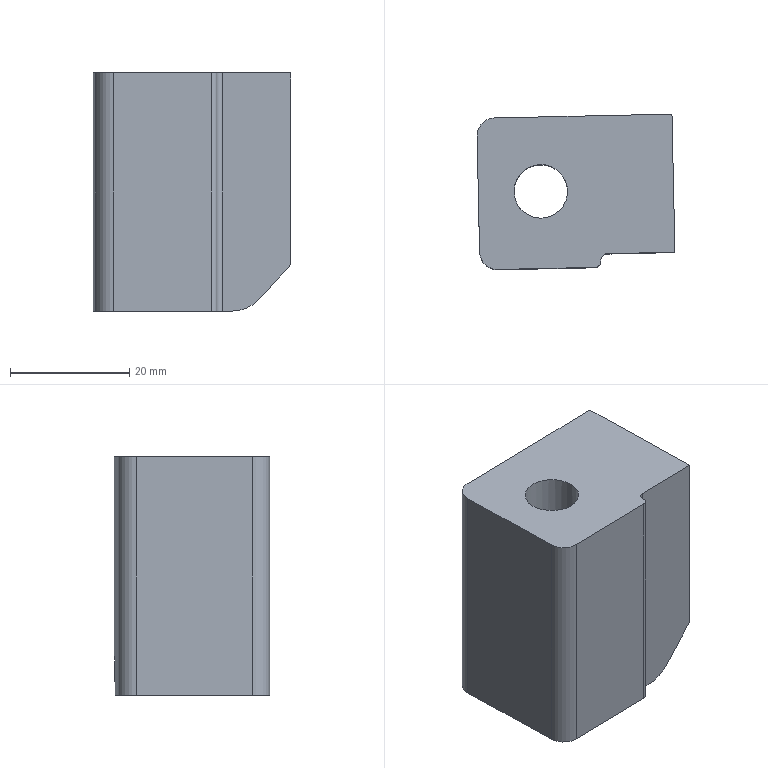Part | NX | features PS-18 2 | 1 solid | 17 faces | box 33.246 x 26.101 x 40 mm | volume 27415 mm3 | plane 10 | cylinder 7 | commonest cylinder face diameters 6.02 x2 1.98 x1 2.02 x1 9 x1 12 x1 14.5 x1
STEP:
#1=CARTESIAN_POINT('',(3013.955,-811.524,860.716));
#2=VERTEX_POINT('',#1);
#3=CARTESIAN_POINT('',(3006.705,-811.524,860.716));
#4=DIRECTION('',(0.,0.,1.));
#5=DIRECTION('',(1.,0.,0.));
#6=AXIS2_PLACEMENT_3D('',#3,#4,#5);
#7=CIRCLE('',#6,7.25);
#8=EDGE_CURVE('',#2,#2,#7,.T.);
#9=ORIENTED_EDGE('',*,*,#8,.T.);
#10=EDGE_LOOP('',(#9));
#11=FACE_BOUND('',#10,.T.);
#12=CARTESIAN_POINT('',(3016.814,-823.258,860.716));
#13=VERTEX_POINT('',#12);
#14=CARTESIAN_POINT('',(3016.809,-823.002,860.716));
#15=VERTEX_POINT('',#14);
#16=CARTESIAN_POINT('',(3016.836,-824.258,860.716));
#17=DIRECTION('',(0.0214,-0.9998,0.));
#18=VECTOR('',#17,1000.);
#19=LINE('',#16,#18);
#20=EDGE_CURVE('',#13,#15,#19,.F.);
#21=ORIENTED_EDGE('',*,*,#20,.F.);
#22=CARTESIAN_POINT('',(3015.826,-824.29,860.716));
#23=VERTEX_POINT('',#22);
#24=CARTESIAN_POINT('',(3015.804,-823.28,860.716));
#25=DIRECTION('',(0.,0.,1.));
#26=DIRECTION('',(1.,0.,0.));
#27=AXIS2_PLACEMENT_3D('',#24,#25,#26);
#28=CIRCLE('',#27,1.01);
#29=EDGE_CURVE('',#13,#23,#28,.F.);
#30=ORIENTED_EDGE('',*,*,#29,.T.);
#31=CARTESIAN_POINT('',(2999.484,-824.639,860.716));
#32=VERTEX_POINT('',#31);
#33=CARTESIAN_POINT('',(2866.42,-827.487,860.716));
#34=DIRECTION('',(0.9998,0.0214,0.));
#35=VECTOR('',#34,1000.);
#36=LINE('',#33,#35);
#37=EDGE_CURVE('',#23,#32,#36,.F.);
#38=ORIENTED_EDGE('',*,*,#37,.T.);
#39=CARTESIAN_POINT('',(2996.411,-821.694,860.716));
#40=VERTEX_POINT('',#39);
#41=CARTESIAN_POINT('',(2999.42,-821.63,860.716));
#42=DIRECTION('',(0.,0.,1.));
#43=DIRECTION('',(1.,0.,0.));
#44=AXIS2_PLACEMENT_3D('',#41,#42,#43);
#45=CIRCLE('',#44,3.01);
#46=EDGE_CURVE('',#32,#40,#45,.F.);
#47=ORIENTED_EDGE('',*,*,#46,.T.);
#48=CARTESIAN_POINT('',(2995.994,-802.251,860.716));
#49=VERTEX_POINT('',#48);
#50=CARTESIAN_POINT('',(2995.93,-799.251,860.716));
#51=DIRECTION('',(0.0214,-0.9998,0.));
#52=VECTOR('',#51,1000.);
#53=LINE('',#50,#52);
#54=EDGE_CURVE('',#49,#40,#53,.T.);
#55=ORIENTED_EDGE('',*,*,#54,.F.);
#56=CARTESIAN_POINT('',(2998.939,-799.177,860.716));
#57=VERTEX_POINT('',#56);
#58=CARTESIAN_POINT('',(2999.004,-802.186,860.716));
#59=DIRECTION('',(0.,0.,1.));
#60=DIRECTION('',(1.,0.,0.));
#61=AXIS2_PLACEMENT_3D('',#58,#59,#60);
#62=CIRCLE('',#61,3.01);
#63=EDGE_CURVE('',#49,#57,#62,.F.);
#64=ORIENTED_EDGE('',*,*,#63,.T.);
#65=CARTESIAN_POINT('',(3018.912,-798.75,860.716));
#66=VERTEX_POINT('',#65);
#67=CARTESIAN_POINT('',(3028.943,-798.535,860.716));
#68=DIRECTION('',(-0.9998,-0.0214,0.));
#69=VECTOR('',#68,1000.);
#70=LINE('',#67,#69);
#71=EDGE_CURVE('',#57,#66,#70,.F.);
#72=ORIENTED_EDGE('',*,*,#71,.T.);
#73=CARTESIAN_POINT('',(3019.409,-821.956,860.716));
#74=VERTEX_POINT('',#73);
#75=CARTESIAN_POINT('',(3023.131,-995.847,860.716));
#76=DIRECTION('',(0.0214,-0.9998,0.));
#77=VECTOR('',#76,1000.);
#78=LINE('',#75,#77);
#79=EDGE_CURVE('',#66,#74,#78,.T.);
#80=ORIENTED_EDGE('',*,*,#79,.T.);
#81=CARTESIAN_POINT('',(3017.777,-821.991,860.716));
#82=VERTEX_POINT('',#81);
#83=CARTESIAN_POINT('',(2866.372,-825.232,860.716));
#84=DIRECTION('',(0.9998,0.0214,0.));
#85=VECTOR('',#84,1000.);
#86=LINE('',#83,#85);
#87=EDGE_CURVE('',#74,#82,#86,.F.);
#88=ORIENTED_EDGE('',*,*,#87,.T.);
#89=CARTESIAN_POINT('',(3017.798,-822.981,860.716));
#90=DIRECTION('',(0.,0.,1.));
#91=DIRECTION('',(1.,0.,0.));
#92=AXIS2_PLACEMENT_3D('',#89,#90,#91);
#93=CIRCLE('',#92,0.99);
#94=EDGE_CURVE('',#82,#15,#93,.T.);
#95=ORIENTED_EDGE('',*,*,#94,.T.);
#96=EDGE_LOOP('',(#21,#30,#38,#47,#55,#64,#72,#80,#88,#95));
#97=FACE_BOUND('',#96,.T.);
#98=CARTESIAN_POINT('',(2870.094,-999.122,860.716));
#99=DIRECTION('',(0.,0.,1.));
#100=DIRECTION('',(0.,1.,0.));
#101=AXIS2_PLACEMENT_3D('',#98,#99,#100);
#102=PLANE('',#101);
#103=ADVANCED_FACE('',(#11,#97),#102,.F.);
#104=ORIENTED_EDGE('',*,*,#20,.T.);
#105=CARTESIAN_POINT('',(3016.809,-823.002,900.716));
#106=VERTEX_POINT('',#105);
#107=CARTESIAN_POINT('',(3016.809,-823.002,880.716));
#108=DIRECTION('',(0.,0.,1.));
#109=VECTOR('',#108,1000.);
#110=LINE('',#107,#109);
#111=EDGE_CURVE('',#15,#106,#110,.T.);
#112=ORIENTED_EDGE('',*,*,#111,.T.);
#113=CARTESIAN_POINT('',(3016.814,-823.258,900.716));
#114=VERTEX_POINT('',#113);
#115=CARTESIAN_POINT('',(3016.836,-824.258,900.716));
#116=DIRECTION('',(0.0214,-0.9998,0.));
#117=VECTOR('',#116,1000.);
#118=LINE('',#115,#117);
#119=EDGE_CURVE('',#106,#114,#118,.T.);
#120=ORIENTED_EDGE('',*,*,#119,.T.);
#121=CARTESIAN_POINT('',(3016.814,-823.258,880.716));
#122=DIRECTION('',(0.,0.,1.));
#123=VECTOR('',#122,1000.);
#124=LINE('',#121,#123);
#125=EDGE_CURVE('',#114,#13,#124,.F.);
#126=ORIENTED_EDGE('',*,*,#125,.T.);
#127=EDGE_LOOP('',(#104,#112,#120,#126));
#128=FACE_BOUND('',#127,.T.);
#129=CARTESIAN_POINT('',(3016.836,-824.258,880.716));
#130=DIRECTION('',(0.9998,0.0214,0.));
#131=DIRECTION('',(0.,0.,1.));
#132=AXIS2_PLACEMENT_3D('',#129,#130,#131);
#133=PLANE('',#132);
#134=ADVANCED_FACE('',(#128),#133,.T.);
#135=ORIENTED_EDGE('',*,*,#37,.F.);
#136=CARTESIAN_POINT('',(3015.826,-824.29,900.716));
#137=VERTEX_POINT('',#136);
#138=CARTESIAN_POINT('',(3015.826,-824.29,880.716));
#139=DIRECTION('',(0.,0.,-1.));
#140=VECTOR('',#139,1000.);
#141=LINE('',#138,#140);
#142=EDGE_CURVE('',#23,#137,#141,.F.);
#143=ORIENTED_EDGE('',*,*,#142,.T.);
#144=CARTESIAN_POINT('',(2999.484,-824.639,900.716));
#145=VERTEX_POINT('',#144);
#146=CARTESIAN_POINT('',(2881.104,-827.173,900.716));
#147=DIRECTION('',(0.9998,0.0214,0.));
#148=VECTOR('',#147,1000.);
#149=LINE('',#146,#148);
#150=EDGE_CURVE('',#145,#137,#149,.T.);
#151=ORIENTED_EDGE('',*,*,#150,.F.);
#152=CARTESIAN_POINT('',(2999.484,-824.639,880.716));
#153=DIRECTION('',(0.,0.,-1.));
#154=VECTOR('',#153,1000.);
#155=LINE('',#152,#154);
#156=EDGE_CURVE('',#145,#32,#155,.T.);
#157=ORIENTED_EDGE('',*,*,#156,.T.);
#158=EDGE_LOOP('',(#135,#143,#151,#157));
#159=FACE_BOUND('',#158,.T.);
#160=CARTESIAN_POINT('',(2996.485,-824.703,880.716));
#161=DIRECTION('',(0.0214,-0.9998,0.));
#162=DIRECTION('',(0.,0.,-1.));
#163=AXIS2_PLACEMENT_3D('',#160,#161,#162);
#164=PLANE('',#163);
#165=ADVANCED_FACE('',(#159),#164,.T.);
#166=CARTESIAN_POINT('',(2995.994,-802.251,900.716));
#167=VERTEX_POINT('',#166);
#168=CARTESIAN_POINT('',(2996.411,-821.694,900.716));
#169=VERTEX_POINT('',#168);
#170=CARTESIAN_POINT('',(2995.295,-769.576,900.716));
#171=DIRECTION('',(-0.0214,0.9998,0.));
#172=VECTOR('',#171,1000.);
#173=LINE('',#170,#172);
#174=EDGE_CURVE('',#167,#169,#173,.F.);
#175=ORIENTED_EDGE('',*,*,#174,.F.);
#176=CARTESIAN_POINT('',(2995.994,-802.251,888.716));
#177=DIRECTION('',(0.,0.,1.));
#178=VECTOR('',#177,1000.);
#179=LINE('',#176,#178);
#180=EDGE_CURVE('',#167,#49,#179,.F.);
#181=ORIENTED_EDGE('',*,*,#180,.T.);
#182=ORIENTED_EDGE('',*,*,#54,.T.);
#183=CARTESIAN_POINT('',(2996.411,-821.694,888.716));
#184=DIRECTION('',(0.,0.,1.));
#185=VECTOR('',#184,1000.);
#186=LINE('',#183,#185);
#187=EDGE_CURVE('',#40,#169,#186,.T.);
#188=ORIENTED_EDGE('',*,*,#187,.T.);
#189=EDGE_LOOP('',(#175,#181,#182,#188));
#190=FACE_BOUND('',#189,.T.);
#191=CARTESIAN_POINT('',(2995.93,-799.251,888.716));
#192=DIRECTION('',(0.9998,0.0214,0.));
#193=DIRECTION('',(0.,0.,1.));
#194=AXIS2_PLACEMENT_3D('',#191,#192,#193);
#195=PLANE('',#194);
#196=ADVANCED_FACE('',(#190),#195,.F.);
#197=ORIENTED_EDGE('',*,*,#71,.F.);
#198=CARTESIAN_POINT('',(2998.939,-799.177,900.716));
#199=VERTEX_POINT('',#198);
#200=CARTESIAN_POINT('',(2998.939,-799.177,888.716));
#201=DIRECTION('',(0.,0.,-1.));
#202=VECTOR('',#201,1000.);
#203=LINE('',#200,#202);
#204=EDGE_CURVE('',#57,#199,#203,.F.);
#205=ORIENTED_EDGE('',*,*,#204,.T.);
#206=CARTESIAN_POINT('',(3020.228,-798.721,900.716));
#207=VERTEX_POINT('',#206);
#208=CARTESIAN_POINT('',(2880.559,-801.711,900.716));
#209=DIRECTION('',(0.9998,0.0214,0.));
#210=VECTOR('',#209,1000.);
#211=LINE('',#208,#210);
#212=EDGE_CURVE('',#199,#207,#211,.T.);
#213=ORIENTED_EDGE('',*,*,#212,.T.);
#214=CARTESIAN_POINT('',(3026.717,-798.583,900.716));
#215=VERTEX_POINT('',#214);
#216=CARTESIAN_POINT('',(2880.559,-801.711,900.716));
#217=DIRECTION('',(0.9998,0.0214,0.));
#218=VECTOR('',#217,1000.);
#219=LINE('',#216,#218);
#220=EDGE_CURVE('',#207,#215,#219,.T.);
#221=ORIENTED_EDGE('',*,*,#220,.T.);
#222=CARTESIAN_POINT('',(3028.743,-798.539,900.716));
#223=VERTEX_POINT('',#222);
#224=CARTESIAN_POINT('',(2880.559,-801.711,900.716));
#225=DIRECTION('',(0.9998,0.0214,0.));
#226=VECTOR('',#225,1000.);
#227=LINE('',#224,#226);
#228=EDGE_CURVE('',#215,#223,#227,.T.);
#229=ORIENTED_EDGE('',*,*,#228,.T.);
#230=CARTESIAN_POINT('',(3028.743,-798.539,868.5));
#231=VERTEX_POINT('',#230);
#232=CARTESIAN_POINT('',(3028.743,-798.539,888.716));
#233=DIRECTION('',(0.,0.,1.));
#234=VECTOR('',#233,1000.);
#235=LINE('',#232,#234);
#236=EDGE_CURVE('',#223,#231,#235,.F.);
#237=ORIENTED_EDGE('',*,*,#236,.T.);
#238=CARTESIAN_POINT('',(3023.313,-798.655,862.638));
#239=VERTEX_POINT('',#238);
#240=CARTESIAN_POINT('',(3024.151,-798.637,863.544));
#241=DIRECTION('',(0.6795,0.01454,0.7335));
#242=VECTOR('',#241,1000.);
#243=LINE('',#240,#242);
#244=EDGE_CURVE('',#231,#239,#243,.F.);
#245=ORIENTED_EDGE('',*,*,#244,.T.);
#246=CARTESIAN_POINT('',(3018.912,-798.75,866.716));
#247=DIRECTION('',(0.0214,-0.9998,0.));
#248=DIRECTION('',(0.9998,0.0214,0.));
#249=AXIS2_PLACEMENT_3D('',#246,#247,#248);
#250=CIRCLE('',#249,6.);
#251=EDGE_CURVE('',#239,#66,#250,.F.);
#252=ORIENTED_EDGE('',*,*,#251,.T.);
#253=EDGE_LOOP('',(#197,#205,#213,#221,#229,#237,#245,#252));
#254=FACE_BOUND('',#253,.T.);
#255=CARTESIAN_POINT('',(3028.943,-798.535,888.716));
#256=DIRECTION('',(0.0214,-0.9998,0.));
#257=DIRECTION('',(0.,0.,1.));
#258=AXIS2_PLACEMENT_3D('',#255,#256,#257);
#259=PLANE('',#258);
#260=ADVANCED_FACE('',(#254),#259,.F.);
#261=ORIENTED_EDGE('',*,*,#251,.F.);
#262=CARTESIAN_POINT('',(3023.809,-821.862,862.638));
#263=VERTEX_POINT('',#262);
#264=CARTESIAN_POINT('',(3023.521,-808.389,862.638));
#265=DIRECTION('',(0.0214,-0.9998,0.));
#266=VECTOR('',#265,1000.);
#267=LINE('',#264,#266);
#268=EDGE_CURVE('',#263,#239,#267,.F.);
#269=ORIENTED_EDGE('',*,*,#268,.F.);
#270=CARTESIAN_POINT('',(3019.409,-821.956,866.716));
#271=DIRECTION('',(0.0214,-0.9998,0.));
#272=DIRECTION('',(0.9998,0.0214,0.));
#273=AXIS2_PLACEMENT_3D('',#270,#271,#272);
#274=CIRCLE('',#273,6.);
#275=EDGE_CURVE('',#74,#263,#274,.T.);
#276=ORIENTED_EDGE('',*,*,#275,.F.);
#277=ORIENTED_EDGE('',*,*,#79,.F.);
#278=EDGE_LOOP('',(#261,#269,#276,#277));
#279=FACE_BOUND('',#278,.T.);
#280=CARTESIAN_POINT('',(3023.131,-995.847,866.716));
#281=DIRECTION('',(0.0214,-0.9998,0.));
#282=DIRECTION('',(0.9998,0.0214,0.));
#283=AXIS2_PLACEMENT_3D('',#280,#281,#282);
#284=CYLINDRICAL_SURFACE('',#283,6.);
#285=ADVANCED_FACE('',(#279),#284,.T.);
#286=CARTESIAN_POINT('',(3006.705,-816.024,900.716));
#287=VERTEX_POINT('',#286);
#288=CARTESIAN_POINT('',(3006.705,-811.524,900.716));
#289=DIRECTION('',(0.,0.,1.));
#290=DIRECTION('',(0.,-1.,0.));
#291=AXIS2_PLACEMENT_3D('',#288,#289,#290);
#292=CIRCLE('',#291,4.5);
#293=EDGE_CURVE('',#287,#287,#292,.F.);
#294=ORIENTED_EDGE('',*,*,#293,.T.);
#295=EDGE_LOOP('',(#294));
#296=FACE_BOUND('',#295,.T.);
#297=ORIENTED_EDGE('',*,*,#150,.T.);
#298=CARTESIAN_POINT('',(3015.804,-823.28,900.716));
#299=DIRECTION('',(0.,0.,1.));
#300=DIRECTION('',(0.,-1.,0.));
#301=AXIS2_PLACEMENT_3D('',#298,#299,#300);
#302=CIRCLE('',#301,1.01);
#303=EDGE_CURVE('',#137,#114,#302,.T.);
#304=ORIENTED_EDGE('',*,*,#303,.T.);
#305=ORIENTED_EDGE('',*,*,#119,.F.);
#306=CARTESIAN_POINT('',(3017.777,-821.991,900.716));
#307=VERTEX_POINT('',#306);
#308=CARTESIAN_POINT('',(3017.798,-822.981,900.716));
#309=DIRECTION('',(0.,0.,1.));
#310=DIRECTION('',(0.,-1.,0.));
#311=AXIS2_PLACEMENT_3D('',#308,#309,#310);
#312=CIRCLE('',#311,0.99);
#313=EDGE_CURVE('',#106,#307,#312,.F.);
#314=ORIENTED_EDGE('',*,*,#313,.T.);
#315=CARTESIAN_POINT('',(3029.24,-821.746,900.716));
#316=VERTEX_POINT('',#315);
#317=CARTESIAN_POINT('',(2881.056,-824.918,900.716));
#318=DIRECTION('',(0.9998,0.0214,0.));
#319=VECTOR('',#318,1000.);
#320=LINE('',#317,#319);
#321=EDGE_CURVE('',#307,#316,#320,.T.);
#322=ORIENTED_EDGE('',*,*,#321,.T.);
#323=CARTESIAN_POINT('',(3028.108,-768.874,900.716));
#324=DIRECTION('',(0.0214,-0.9998,0.));
#325=VECTOR('',#324,1000.);
#326=LINE('',#323,#325);
#327=EDGE_CURVE('',#316,#223,#326,.F.);
#328=ORIENTED_EDGE('',*,*,#327,.T.);
#329=ORIENTED_EDGE('',*,*,#228,.F.);
#330=ORIENTED_EDGE('',*,*,#220,.F.);
#331=ORIENTED_EDGE('',*,*,#212,.F.);
#332=CARTESIAN_POINT('',(2999.004,-802.186,900.716));
#333=DIRECTION('',(0.,0.,1.));
#334=DIRECTION('',(0.,-1.,0.));
#335=AXIS2_PLACEMENT_3D('',#332,#333,#334);
#336=CIRCLE('',#335,3.01);
#337=EDGE_CURVE('',#199,#167,#336,.T.);
#338=ORIENTED_EDGE('',*,*,#337,.T.);
#339=ORIENTED_EDGE('',*,*,#174,.T.);
#340=CARTESIAN_POINT('',(2999.42,-821.63,900.716));
#341=DIRECTION('',(0.,0.,1.));
#342=DIRECTION('',(0.,-1.,0.));
#343=AXIS2_PLACEMENT_3D('',#340,#341,#342);
#344=CIRCLE('',#343,3.01);
#345=EDGE_CURVE('',#169,#145,#344,.T.);
#346=ORIENTED_EDGE('',*,*,#345,.T.);
#347=EDGE_LOOP('',(#297,#304,#305,#314,#322,#328,#329,#330,#331,#338,#339,#346));
#348=FACE_BOUND('',#347,.T.);
#349=CARTESIAN_POINT('',(2879.924,-772.046,900.716));
#350=DIRECTION('',(0.,0.,1.));
#351=DIRECTION('',(0.9976,0.06975,0.));
#352=AXIS2_PLACEMENT_3D('',#349,#350,#351);
#353=PLANE('',#352);
#354=ADVANCED_FACE('',(#296,#348),#353,.T.);
#355=CARTESIAN_POINT('',(3029.24,-821.746,868.5));
#356=VERTEX_POINT('',#355);
#357=CARTESIAN_POINT('',(3035.421,-821.614,875.173));
#358=DIRECTION('',(-0.6795,-0.01454,-0.7335));
#359=VECTOR('',#358,1000.);
#360=LINE('',#357,#359);
#361=EDGE_CURVE('',#263,#356,#360,.F.);
#362=ORIENTED_EDGE('',*,*,#361,.F.);
#363=ORIENTED_EDGE('',*,*,#268,.T.);
#364=ORIENTED_EDGE('',*,*,#244,.F.);
#365=CARTESIAN_POINT('',(3028.99,-810.086,868.5));
#366=DIRECTION('',(-0.0214,0.9998,0.));
#367=VECTOR('',#366,1000.);
#368=LINE('',#365,#367);
#369=EDGE_CURVE('',#356,#231,#368,.T.);
#370=ORIENTED_EDGE('',*,*,#369,.F.);
#371=EDGE_LOOP('',(#362,#363,#364,#370));
#372=FACE_BOUND('',#371,.T.);
#373=CARTESIAN_POINT('',(3024.36,-808.371,863.544));
#374=DIRECTION('',(-0.7334,-0.0157,0.6797));
#375=DIRECTION('',(0.6797,0.,0.7334));
#376=AXIS2_PLACEMENT_3D('',#373,#374,#375);
#377=PLANE('',#376);
#378=ADVANCED_FACE('',(#372),#377,.F.);
#379=ORIENTED_EDGE('',*,*,#321,.F.);
#380=CARTESIAN_POINT('',(3017.777,-821.991,880.716));
#381=DIRECTION('',(0.,0.,1.));
#382=VECTOR('',#381,1000.);
#383=LINE('',#380,#382);
#384=EDGE_CURVE('',#307,#82,#383,.F.);
#385=ORIENTED_EDGE('',*,*,#384,.T.);
#386=ORIENTED_EDGE('',*,*,#87,.F.);
#387=ORIENTED_EDGE('',*,*,#275,.T.);
#388=ORIENTED_EDGE('',*,*,#361,.T.);
#389=CARTESIAN_POINT('',(3029.24,-821.746,888.716));
#390=DIRECTION('',(0.,0.,1.));
#391=VECTOR('',#390,1000.);
#392=LINE('',#389,#391);
#393=EDGE_CURVE('',#316,#356,#392,.F.);
#394=ORIENTED_EDGE('',*,*,#393,.F.);
#395=EDGE_LOOP('',(#379,#385,#386,#387,#388,#394));
#396=FACE_BOUND('',#395,.T.);
#397=CARTESIAN_POINT('',(3029.44,-821.742,880.716));
#398=DIRECTION('',(0.0214,-0.9998,0.));
#399=DIRECTION('',(0.,0.,1.));
#400=AXIS2_PLACEMENT_3D('',#397,#398,#399);
#401=PLANE('',#400);
#402=ADVANCED_FACE('',(#396),#401,.T.);
#403=ORIENTED_EDGE('',*,*,#393,.T.);
#404=ORIENTED_EDGE('',*,*,#369,.T.);
#405=ORIENTED_EDGE('',*,*,#236,.F.);
#406=ORIENTED_EDGE('',*,*,#327,.F.);
#407=EDGE_LOOP('',(#403,#404,#405,#406));
#408=FACE_BOUND('',#407,.T.);
#409=CARTESIAN_POINT('',(3028.99,-810.086,888.716));
#410=DIRECTION('',(-0.9998,-0.0214,0.));
#411=DIRECTION('',(0.0214,-0.9998,0.));
#412=AXIS2_PLACEMENT_3D('',#409,#410,#411);
#413=PLANE('',#412);
#414=ADVANCED_FACE('',(#408),#413,.F.);
#415=CARTESIAN_POINT('',(3013.954,-811.369,875.716));
#416=VERTEX_POINT('',#415);
#417=CARTESIAN_POINT('',(3006.705,-811.524,875.716));
#418=DIRECTION('',(0.,0.,-1.));
#419=DIRECTION('',(0.9998,0.0214,0.));
#420=AXIS2_PLACEMENT_3D('',#417,#418,#419);
#421=CIRCLE('',#420,7.25);
#422=EDGE_CURVE('',#416,#416,#421,.F.);
#423=ORIENTED_EDGE('',*,*,#422,.T.);
#424=EDGE_LOOP('',(#423));
#425=FACE_BOUND('',#424,.T.);
#426=ORIENTED_EDGE('',*,*,#8,.F.);
#427=EDGE_LOOP('',(#426));
#428=FACE_BOUND('',#427,.T.);
#429=CARTESIAN_POINT('',(3006.705,-811.524,875.716));
#430=DIRECTION('',(0.,0.,-1.));
#431=DIRECTION('',(-1.,0.,0.));
#432=AXIS2_PLACEMENT_3D('',#429,#430,#431);
#433=CYLINDRICAL_SURFACE('',#432,7.25);
#434=ADVANCED_FACE('',(#425,#428),#433,.F.);
#435=CARTESIAN_POINT('',(3002.205,-811.524,875.716));
#436=VERTEX_POINT('',#435);
#437=CARTESIAN_POINT('',(3006.705,-811.524,875.716));
#438=DIRECTION('',(0.,0.,-1.));
#439=DIRECTION('',(-1.,0.,0.));
#440=AXIS2_PLACEMENT_3D('',#437,#438,#439);
#441=CIRCLE('',#440,4.5);
#442=EDGE_CURVE('',#436,#436,#441,.T.);
#443=ORIENTED_EDGE('',*,*,#442,.T.);
#444=EDGE_LOOP('',(#443));
#445=FACE_BOUND('',#444,.T.);
#446=ORIENTED_EDGE('',*,*,#293,.F.);
#447=EDGE_LOOP('',(#446));
#448=FACE_BOUND('',#447,.T.);
#449=CARTESIAN_POINT('',(3006.705,-811.524,901.716));
#450=DIRECTION('',(0.,0.,-1.));
#451=DIRECTION('',(-1.,0.,0.));
#452=AXIS2_PLACEMENT_3D('',#449,#450,#451);
#453=CYLINDRICAL_SURFACE('',#452,4.5);
#454=ADVANCED_FACE('',(#445,#448),#453,.F.);
#455=ORIENTED_EDGE('',*,*,#442,.F.);
#456=EDGE_LOOP('',(#455));
#457=FACE_BOUND('',#456,.T.);
#458=ORIENTED_EDGE('',*,*,#422,.F.);
#459=EDGE_LOOP('',(#458));
#460=FACE_BOUND('',#459,.T.);
#461=CARTESIAN_POINT('',(3006.705,-811.524,875.716));
#462=DIRECTION('',(0.,0.,-1.));
#463=DIRECTION('',(-1.,0.,0.));
#464=AXIS2_PLACEMENT_3D('',#461,#462,#463);
#465=PLANE('',#464);
#466=ADVANCED_FACE('',(#457,#460),#465,.T.);
#467=ORIENTED_EDGE('',*,*,#337,.F.);
#468=ORIENTED_EDGE('',*,*,#204,.F.);
#469=ORIENTED_EDGE('',*,*,#63,.F.);
#470=ORIENTED_EDGE('',*,*,#180,.F.);
#471=EDGE_LOOP('',(#467,#468,#469,#470));
#472=FACE_BOUND('',#471,.T.);
#473=CARTESIAN_POINT('',(2999.004,-802.186,888.716));
#474=DIRECTION('',(0.,0.,-1.));
#475=DIRECTION('',(-1.,0.,0.));
#476=AXIS2_PLACEMENT_3D('',#473,#474,#475);
#477=CYLINDRICAL_SURFACE('',#476,3.01);
#478=ADVANCED_FACE('',(#472),#477,.T.);
#479=ORIENTED_EDGE('',*,*,#345,.F.);
#480=ORIENTED_EDGE('',*,*,#187,.F.);
#481=ORIENTED_EDGE('',*,*,#46,.F.);
#482=ORIENTED_EDGE('',*,*,#156,.F.);
#483=EDGE_LOOP('',(#479,#480,#481,#482));
#484=FACE_BOUND('',#483,.T.);
#485=CARTESIAN_POINT('',(2999.42,-821.63,880.716));
#486=DIRECTION('',(0.,0.,1.));
#487=DIRECTION('',(1.,0.,0.));
#488=AXIS2_PLACEMENT_3D('',#485,#486,#487);
#489=CYLINDRICAL_SURFACE('',#488,3.01);
#490=ADVANCED_FACE('',(#484),#489,.T.);
#491=ORIENTED_EDGE('',*,*,#313,.F.);
#492=ORIENTED_EDGE('',*,*,#111,.F.);
#493=ORIENTED_EDGE('',*,*,#94,.F.);
#494=ORIENTED_EDGE('',*,*,#384,.F.);
#495=EDGE_LOOP('',(#491,#492,#493,#494));
#496=FACE_BOUND('',#495,.T.);
#497=CARTESIAN_POINT('',(3017.798,-822.981,880.716));
#498=DIRECTION('',(0.,0.,1.));
#499=DIRECTION('',(1.,0.,0.));
#500=AXIS2_PLACEMENT_3D('',#497,#498,#499);
#501=CYLINDRICAL_SURFACE('',#500,0.99);
#502=ADVANCED_FACE('',(#496),#501,.F.);
#503=ORIENTED_EDGE('',*,*,#303,.F.);
#504=ORIENTED_EDGE('',*,*,#142,.F.);
#505=ORIENTED_EDGE('',*,*,#29,.F.);
#506=ORIENTED_EDGE('',*,*,#125,.F.);
#507=EDGE_LOOP('',(#503,#504,#505,#506));
#508=FACE_BOUND('',#507,.T.);
#509=CARTESIAN_POINT('',(3015.804,-823.28,880.716));
#510=DIRECTION('',(0.,0.,-1.));
#511=DIRECTION('',(-1.,0.,0.));
#512=AXIS2_PLACEMENT_3D('',#509,#510,#511);
#513=CYLINDRICAL_SURFACE('',#512,1.01);
#514=ADVANCED_FACE('',(#508),#513,.T.);
#515=CLOSED_SHELL('',(#103,#134,#165,#196,#260,#285,#354,#378,#402,#414,#434,#454,#466,#478,#490,#502,#514));
#516=MANIFOLD_SOLID_BREP('',#515);
#517=(LENGTH_UNIT()NAMED_UNIT(*)SI_UNIT(.MILLI.,.METRE.));
#518=UNCERTAINTY_MEASURE_WITH_UNIT(LENGTH_MEASURE(0.00001),#517,'','');
#519=(NAMED_UNIT(*)PLANE_ANGLE_UNIT()SI_UNIT($,.RADIAN.));
#520=(NAMED_UNIT(*)SI_UNIT($,.STERADIAN.)SOLID_ANGLE_UNIT());
#521=(GEOMETRIC_REPRESENTATION_CONTEXT(3)GLOBAL_UNCERTAINTY_ASSIGNED_CONTEXT((#518))GLOBAL_UNIT_ASSIGNED_CONTEXT((#517,#519,#520))REPRESENTATION_CONTEXT('',''));
#522=ADVANCED_BREP_SHAPE_REPRESENTATION('',(#516),#521);